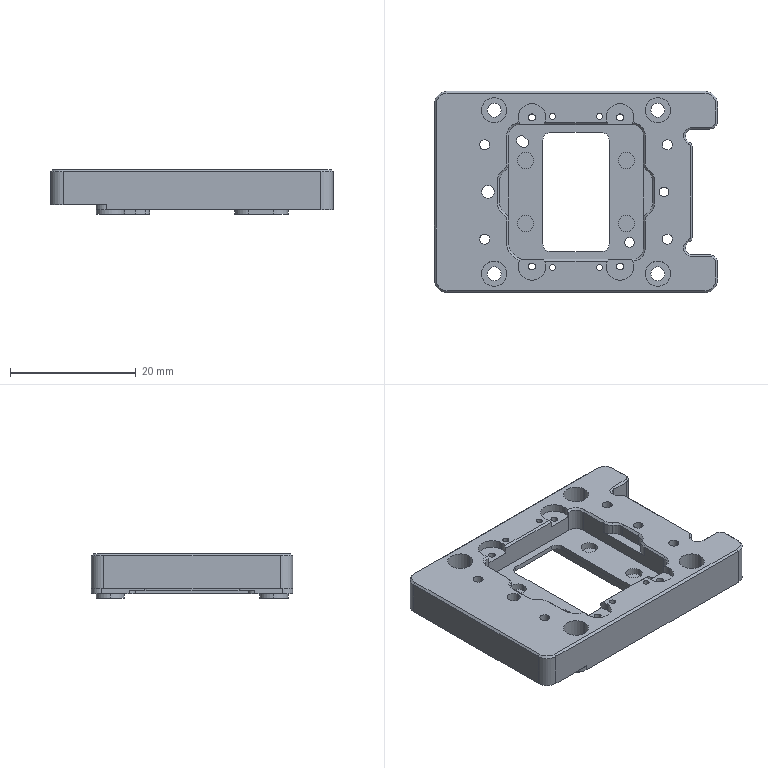NC program | NX | posted with a generic post | part box 45 x 32 x 7.05 mm
Lines 5416 to 5787 of 5787:
(PLANAR_MILL , TOOL : D6A45)
N10722 T01 M6
N10724 G54
N10726 G17 G0 G90 X-0.866 Y17.2 S9500 M3
N10728 G43 Z30. H1
N10730 Z0.5
N10732 G94 G1 Z-1. F1250.
N10734 G3 X0. Y16.7 R1.
N10736 G1 X20.5
N10738 G2 X23.2 Y14. R2.7
N10740 G1 Y11.214
N10742 G2 X21.286 Y9.3 R2.062
N10744 G1 X18.5
N10746 G3 X18.31 Y8.548 R0.4
N10748 G2 X19.2 Y7.053 R1.7
N10750 G1 Y-7.053
N10752 G2 X18.31 Y-8.548 R1.7
N10754 G3 X18.5 Y-9.3 R0.4
N10756 G1 X21.618 Y-9.333
N10758 G2 X23.2 Y-11.214 R2.134
N10760 G1 Y-14.
N10762 G2 X20.5 Y-16.7 R2.7
N10764 G1 X-20.5
N10766 G2 X-23.2 Y-14. R2.7
N10768 G1 Y14.
N10770 G2 X-20.5 Y16.7 R2.7
N10772 G1 X0.
N10774 G3 X0.866 Y17.2 R1.
N10776 G1 Z0.5
N10778 G0 Z30.
(PLANAR_MILL_COPY_1 , TOOL : D6A45)
N10780 X-9.5 Y1.177
N10782 Z0.5
N10784 G1 Z-1.
N10786 G3 X-10. Y0.311 R1.
N10788 G1 Y-8.379
N10790 G3 X-9.707 Y-9.086 R1.
N10792 G1 X-9.086 Y-9.707
N10794 G3 X-8.379 Y-10. R1.
N10796 G1 X9.
N10798 G3 X10. Y-9. R1.
N10800 G1 Y9.
N10802 G3 X9. Y10. R1.
N10804 G1 X-9.
N10806 G3 X-10. Y9. R1.
N10808 G1 Y0.311
N10810 G3 X-9.5 Y-0.555 R1.
N10812 G1 Z0.5
N10814 G0 Z30.
(PLANAR_MILL_COPY_1_COPY , TOOL : D6A45)
N10816 X-10.054 Y2.696
N10818 Z0.5
N10820 G1 Z-1.
N10822 G3 X-11.05 Y2.612 R1.
N10824 X-11.5 Y1.75 R1.05
N10826 G1 Y-1.75
N10828 G3 X-11.05 Y-2.612 R1.05
N10830 G2 X-10. Y-4.622 R2.45
N10832 G3 X-9.5 Y-5.488 R1.
N10834 G1 Z0.5
N10836 G0 Z30.
N10838 X9.5
N10840 Z0.5
N10842 G1 Z-1.
N10844 G3 X10. Y-4.622 R1.
N10846 G2 X11.05 Y-2.612 R2.45
N10848 G3 X11.5 Y-1.75 R1.05
N10850 G1 Y1.75
N10852 G3 X11.05 Y2.612 R1.05
N10854 G2 X10. Y4.622 R2.45
N10856 G3 X9.5 Y5.488 R1.
N10858 G1 Z0.5
N10860 G0 Z30.
(PLANAR_MILL_COPY , TOOL : D6A45)
N10862 X-13.8 Y-12.134
N10864 Z0.2
N10866 G1 Z-0.8
N10868 G3 X-14.3 Y-13. R1.
N10870 X-13. Y-14.3 R1.3
N10872 X-14.3 Y-13. R-1.3
N10874 X-13.8 Y-13.866 R1.
N10876 G1 Z0.2
N10878 G0 Z30.
N10880 X-14.6 Y-7.57
N10882 Z0.2
N10884 G1 X-14.4 Y-7.583 Z0.139
N10886 X-14.417 Y-7.4 Z0.088
N10888 X-14.6 Y-7.417 Z0.037
N10890 X-14.583 Y-7.6 Z-0.014
N10892 X-14.4 Y-7.583 Z-0.065
N10894 X-14.417 Y-7.4 Z-0.116
N10896 X-14.6 Y-7.417 Z-0.167
N10898 X-14.583 Y-7.6 Z-0.217
N10900 X-14.4 Y-7.583 Z-0.268
N10902 X-14.417 Y-7.4 Z-0.319
N10904 X-14.6 Y-7.417 Z-0.37
N10906 X-14.583 Y-7.6 Z-0.421
N10908 X-14.4 Y-7.583 Z-0.472
N10910 X-14.417 Y-7.4 Z-0.523
N10912 X-14.6 Y-7.417 Z-0.574
N10914 X-14.583 Y-7.6 Z-0.625
N10916 X-14.4 Y-7.583 Z-0.676
N10918 X-14.417 Y-7.4 Z-0.727
N10920 X-14.6 Y-7.417 Z-0.778
N10922 Y-7.5 Z-0.8
N10924 G3 X-14.5 Y-7.6 R0.1
N10926 X-14.6 Y-7.5 R-0.1
N10928 G1 Z0.2
N10930 G0 Z30.
N10932 X-13.902 Y-0.267
N10934 Z0.2
N10936 G1 Z-0.8
N10938 G3 X-14.325 Y0. R0.5
N10940 X-14. Y-0.325 R0.325
N10942 X-14.325 Y0. R-0.325
N10944 X-13.902 Y0.267 R0.5
N10946 G1 Z0.2
N10948 G0 Z30.
N10950 X-14.6 Y7.43
N10952 Z0.2
N10954 G1 X-14.4 Y7.417 Z0.139
N10956 X-14.417 Y7.6 Z0.088
N10958 X-14.6 Y7.583 Z0.037
N10960 X-14.583 Y7.4 Z-0.014
N10962 X-14.4 Y7.417 Z-0.065
N10964 X-14.417 Y7.6 Z-0.116
N10966 X-14.6 Y7.583 Z-0.167
N10968 X-14.583 Y7.4 Z-0.217
N10970 X-14.4 Y7.417 Z-0.268
N10972 X-14.417 Y7.6 Z-0.319
N10974 X-14.6 Y7.583 Z-0.37
N10976 X-14.583 Y7.4 Z-0.421
N10978 X-14.4 Y7.417 Z-0.472
N10980 X-14.417 Y7.6 Z-0.523
N10982 X-14.6 Y7.583 Z-0.574
N10984 X-14.583 Y7.4 Z-0.625
N10986 X-14.4 Y7.417 Z-0.676
N10988 X-14.417 Y7.6 Z-0.727
N10990 X-14.6 Y7.583 Z-0.778
N10992 Y7.5 Z-0.8
N10994 G3 X-14.5 Y7.4 R0.1
N10996 X-14.6 Y7.5 R-0.1
N10998 G1 Z0.2
N11000 G0 Z30.
N11002 X-13.8 Y13.866
N11004 Z0.2
N11006 G1 Z-0.8
N11008 G3 X-14.3 Y13. R1.
N11010 X-13. Y11.7 R1.3
N11012 X-14.3 Y13. R-1.3
N11014 X-13.8 Y12.134 R1.
N11016 G1 Z0.2
N11018 G0 Z30.
N11020 X12.2 Y13.866
N11022 Z0.2
N11024 G1 Z-0.8
N11026 G3 X11.7 Y13. R1.
N11028 X13. Y11.7 R1.3
N11030 X11.7 Y13. R-1.3
N11032 X12.2 Y12.134 R1.
N11034 G1 Z0.2
N11036 G0 Z30.
N11038 X14.4 Y7.43
N11040 Z0.2
N11042 G1 X14.6 Y7.417 Z0.139
N11044 X14.583 Y7.6 Z0.088
N11046 X14.4 Y7.583 Z0.037
N11048 X14.417 Y7.4 Z-0.014
N11050 X14.6 Y7.417 Z-0.065
N11052 X14.583 Y7.6 Z-0.116
N11054 X14.4 Y7.583 Z-0.167
N11056 X14.417 Y7.4 Z-0.217
N11058 X14.6 Y7.417 Z-0.268
N11060 X14.583 Y7.6 Z-0.319
N11062 X14.4 Y7.583 Z-0.37
N11064 X14.417 Y7.4 Z-0.421
N11066 X14.6 Y7.417 Z-0.472
N11068 X14.583 Y7.6 Z-0.523
N11070 X14.4 Y7.583 Z-0.574
N11072 X14.417 Y7.4 Z-0.625
N11074 X14.6 Y7.417 Z-0.676
N11076 X14.583 Y7.6 Z-0.727
N11078 X14.4 Y7.583 Z-0.778
N11080 Y7.5 Z-0.8
N11082 G3 X14.5 Y7.4 R0.1
N11084 X14.4 Y7.5 R-0.1
N11086 G1 Z0.2
N11088 G0 Z30.
N11090 X14.004 Y0.075
N11092 Z0.2
N11094 G1 X13.925 Y0.073 Z0.179
N11096 X13.927 Y-0.075 Z0.139
N11098 X14.075 Y-0.073 Z0.099
N11100 X14.073 Y0.075 Z0.059
N11102 X13.925 Y0.073 Z0.019
N11104 X13.927 Y-0.075 Z-0.021
N11106 X14.075 Y-0.073 Z-0.061
N11108 X14.073 Y0.075 Z-0.101
N11110 X13.925 Y0.073 Z-0.141
N11112 X13.927 Y-0.075 Z-0.181
N11114 X14.075 Y-0.073 Z-0.221
N11116 X14.073 Y0.075 Z-0.261
N11118 X13.925 Y0.073 Z-0.301
N11120 X13.927 Y-0.075 Z-0.341
N11122 X14.075 Y-0.073 Z-0.381
N11124 X14.073 Y0.075 Z-0.421
N11126 X13.925 Y0.073 Z-0.461
N11128 X13.927 Y-0.075 Z-0.501
N11130 X14.075 Y-0.073 Z-0.541
N11132 X14.073 Y0.075 Z-0.581
N11134 X13.925 Y0.073 Z-0.62
N11136 X13.927 Y-0.075 Z-0.66
N11138 X14.075 Y-0.073 Z-0.7
N11140 X14.073 Y0.075 Z-0.74
N11142 X13.925 Y0.073 Z-0.78
N11144 Y0. Z-0.8
N11146 G3 X14. Y-0.075 R0.075
N11148 X13.925 Y0. R-0.075
N11150 G1 Z0.2
N11152 G0 Z30.
N11154 X14.4 Y-7.57
N11156 Z0.2
N11158 G1 X14.6 Y-7.583 Z0.139
N11160 X14.583 Y-7.4 Z0.088
N11162 X14.4 Y-7.417 Z0.037
N11164 X14.417 Y-7.6 Z-0.014
N11166 X14.6 Y-7.583 Z-0.065
N11168 X14.583 Y-7.4 Z-0.116
N11170 X14.4 Y-7.417 Z-0.167
N11172 X14.417 Y-7.6 Z-0.217
N11174 X14.6 Y-7.583 Z-0.268
N11176 X14.583 Y-7.4 Z-0.319
N11178 X14.4 Y-7.417 Z-0.37
N11180 X14.417 Y-7.6 Z-0.421
N11182 X14.6 Y-7.583 Z-0.472
N11184 X14.583 Y-7.4 Z-0.523
N11186 X14.4 Y-7.417 Z-0.574
N11188 X14.417 Y-7.6 Z-0.625
N11190 X14.6 Y-7.583 Z-0.676
N11192 X14.583 Y-7.4 Z-0.727
N11194 X14.4 Y-7.417 Z-0.778
N11196 Y-7.5 Z-0.8
N11198 G3 X14.5 Y-7.6 R0.1
N11200 X14.4 Y-7.5 R-0.1
N11202 G1 Z0.2
N11204 G0 Z30.
N11206 X12.2 Y-12.134
N11208 Z0.2
N11210 G1 Z-0.8
N11212 G3 X11.7 Y-13. R1.
N11214 X13. Y-14.3 R1.3
N11216 X11.7 Y-13. R-1.3
N11218 X12.2 Y-13.866 R1.
N11220 G1 Z0.2
N11222 G0 Z30.
(PLANAR_MILL_COPY_COPY , TOOL : D6A45)
N11224 X7.866 Y-11.9
N11226 Z0.2
N11228 G1 Z-0.8
N11230 G3 X7. Y-11.4 R1.
N11232 G1 X5.569
N11234 G3 X8.431 Y-11.4 R-1.5
N11236 G1 X7.
N11238 G3 X6.134 Y-11.9 R1.
N11240 G1 Z0.2
N11242 G0 Z30.
N11244 X-6.134
N11246 Z0.2
N11248 G1 Z-0.8
N11250 G3 X-7. Y-11.4 R1.
N11252 G1 X-8.431 Y-11.399
N11254 G3 X-5.569 Y-11.4 R-1.5
N11256 G1 X-7.
N11258 G3 X-7.866 Y-11.9 R1.
N11260 G1 Z0.2
N11262 G0 Z30.
N11264 Y11.9
N11266 Z0.2
N11268 G1 Z-0.8
N11270 G3 X-7. Y11.4 R1.
N11272 G1 X-5.569
N11274 G3 X-8.431 Y11.4 R-1.5
N11276 G1 X-7.
N11278 G3 X-6.134 Y11.9 R1.
N11280 G1 Z0.2
N11282 G0 Z30.
N11284 X6.134
N11286 Z0.2
N11288 G1 Z-0.8
N11290 G3 X7. Y11.4 R1.
N11292 G1 X8.431
N11294 G3 X5.569 Y11.4 R-1.5
N11296 G1 X7.
N11298 G3 X7.866 Y11.9 R1.
N11300 G1 Z0.2
N11302 G0 Z30.
N11304 M5
(刀补3 , TOOL : D3)
N11306 T17 M6
N11308 G54
N11310 G17 G0 G90 X8.15 Y8.15 S9500 M3
N11312 G43 Z30. H17
N11314 Z-2.85
N11316 G94 G1 Z-3.85 F1000.
N11318 G41 X9.13 Y9.075 D17
N11320 X9.103 Y9.123
N11322 X9.055 Y9.15
N11324 X9.
N11326 X-9.
N11328 G3 X-9.15 Y9. R0.15
N11330 G1 Y-8.379
N11332 X-9.155 Y-8.42
N11334 X-9.139 Y-8.459
N11336 X-9.106 Y-8.485
N11338 X-8.485 Y-9.106
N11340 X-8.459 Y-9.139
N11342 X-8.42 Y-9.155
N11344 X-8.379 Y-9.15
N11346 X9.
N11348 G3 X9.15 Y-9. R0.15
N11350 G1 Y9.
N11352 G3 X9. Y9.15 R0.15
N11354 X8.74 Y9. R0.3
N11356 G1 X8.15 Y7.978
N11358 G40
N11360 X8.116 Y7.884
N11362 Z-2.85
N11364 G0 Z30.
N11366 M5
(刀补21 , TOOL : D1)
N11368 T21 M6
N11370 G54
N11372 G17 G0 G90 X-8.37 Y7.92 S9500 M3
N11374 G43 Z30. H21
N11376 Z-3.85
N11378 G94 G1 Z-5.85 F850.
N11380 G41 X-8.33 Y8.012 D21
N11382 X-8.317 Y8.068
N11384 X-8.305 Y8.104
N11386 X-8.316 Y8.141
N11388 X-8.346 Y8.164
N11390 X-8.528 Y8.335
N11392 G3 X-8.846 Y8.326 R0.225
N11394 X-8.836 Y8.007 R0.225
N11396 G1 X-8.472 Y7.665
N11398 G3 X-8.154 Y7.674 R0.225
N11400 X-8.164 Y7.993 R0.225
N11402 G1 X-8.346 Y8.164
N11404 X-8.371 Y8.192
N11406 X-8.408 Y8.201
N11408 X-8.443 Y8.187
N11410 X-8.498 Y8.17
N11412 G40
N11414 X-8.588 Y8.125
N11416 Z-3.85
N11418 G0 Z30.
N11420 M5
N11422 M2